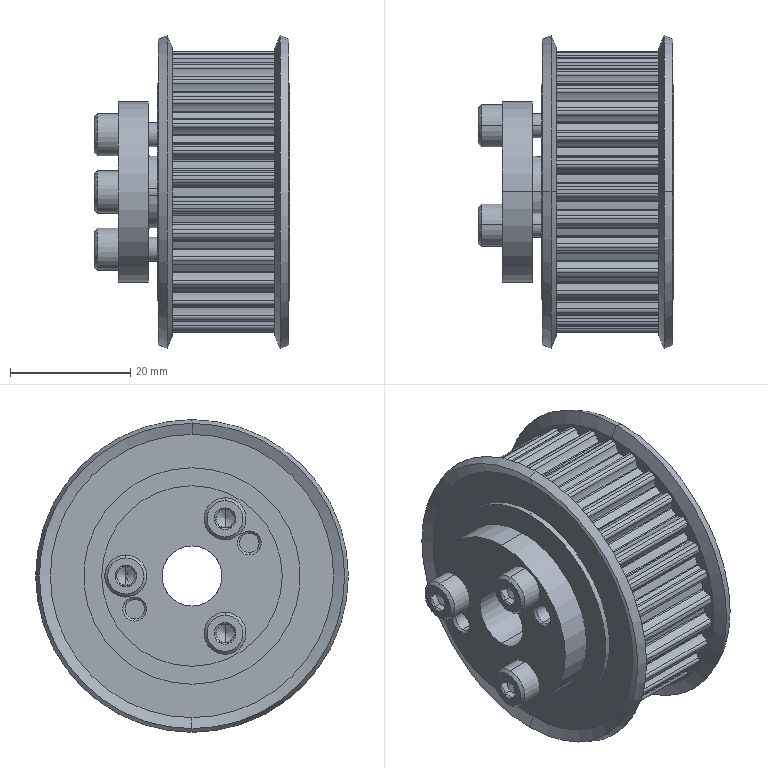Part | NX | features BREP 1 | 1 solid | 408 faces | box 32.5 x 52 x 52 mm | volume 37145 mm3 | cylinder 299 | plane 57 | cone 52 | commonest cylinder face diameters 1.1 x72 0.5 x68 6.55 x64 46.79 x31 43.25 x30 3.242 x10